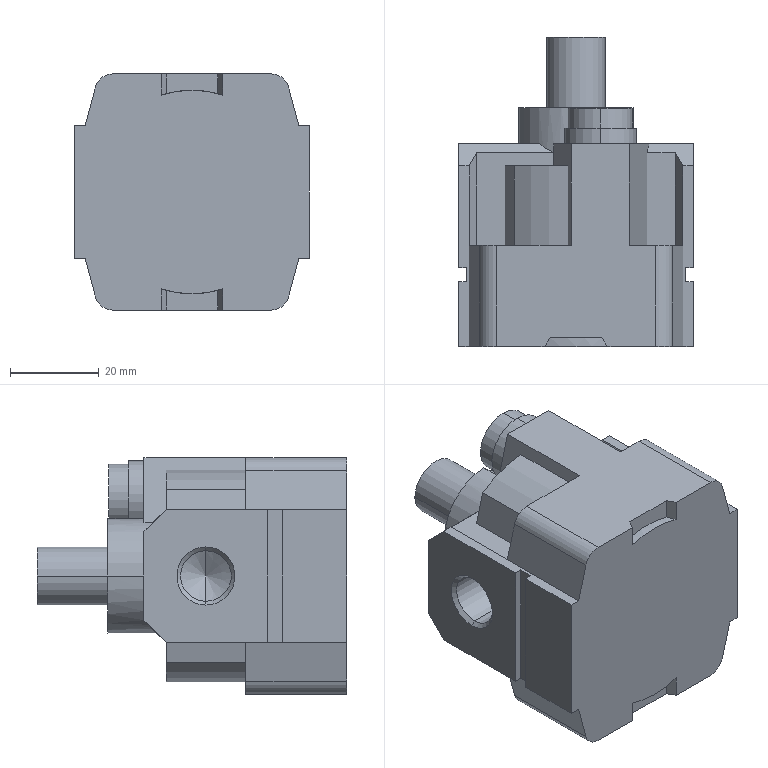Part | STEP file | _AL30-02-A(0)_BODY | 1 solid | 117 faces | box 53 x 69.9 x 53.4 mm | volume 108117 mm3 | plane 63 | cylinder 30 | cone 24 | commonest cylinder face diameters 3.242 x8 8 x4 11.445 x4 26 x3 13.2 x2 14.5 x2